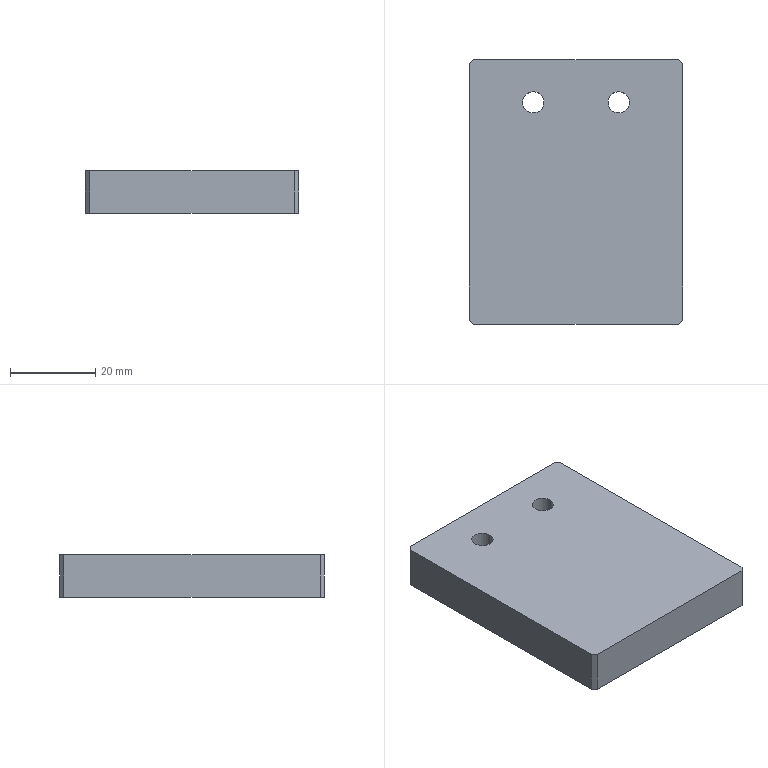Part | STEP file | 2048 Cylinder pad block B | 1 solid | 14 faces | box 50 x 62 x 10 mm | volume 30587 mm3 | plane 10 | cylinder 4 | commonest cylinder face diameters 5 x4
STEP:
#1=CARTESIAN_POINT('',(0.,0.,0.));
#2=DIRECTION('',(0.,0.,1.));
#3=DIRECTION('',(1.,0.,0.));
#4=AXIS2_PLACEMENT_3D('',#1,#2,#3);
#5=CARTESIAN_POINT('',(-7.5,21.,0.));
#6=VERTEX_POINT('',#5);
#7=CARTESIAN_POINT('',(-7.5,21.,10.));
#8=VERTEX_POINT('',#7);
#9=CARTESIAN_POINT('',(-7.5,21.,10.));
#10=DIRECTION('',(0.,0.,1.));
#11=VECTOR('',#10,1.);
#12=LINE('',#9,#11);
#13=CARTESIAN_POINT('',(-10.,21.,10.));
#14=DIRECTION('',(0.,0.,1.));
#15=DIRECTION('',(1.,0.,0.));
#16=AXIS2_PLACEMENT_3D('',#13,#14,#15);
#17=CYLINDRICAL_SURFACE('',#16,2.5);
#18=CARTESIAN_POINT('',(6.283,0.));
#19=DIRECTION('',(0.,1.));
#20=VECTOR('',#19,1.);
#21=LINE('',#18,#20);
#22=(GEOMETRIC_REPRESENTATION_CONTEXT(2)PARAMETRIC_REPRESENTATION_CONTEXT()REPRESENTATION_CONTEXT('',''));
#23=DEFINITIONAL_REPRESENTATION('',(#21),#22);
#24=PCURVE('',#17,#23);
#25=CARTESIAN_POINT('',(-10.,21.,10.));
#26=DIRECTION('',(0.,0.,1.));
#27=DIRECTION('',(1.,0.,0.));
#28=AXIS2_PLACEMENT_3D('',#25,#26,#27);
#29=CYLINDRICAL_SURFACE('',#28,2.5);
#30=CARTESIAN_POINT('',(0.,0.));
#31=DIRECTION('',(0.,1.));
#32=VECTOR('',#31,1.);
#33=LINE('',#30,#32);
#34=(GEOMETRIC_REPRESENTATION_CONTEXT(2)PARAMETRIC_REPRESENTATION_CONTEXT()REPRESENTATION_CONTEXT('',''));
#35=DEFINITIONAL_REPRESENTATION('',(#33),#34);
#36=PCURVE('',#29,#35);
#37=SURFACE_CURVE('',#12,(#24,#36),.PCURVE_S1.);
#38=EDGE_CURVE('',#6,#8,#37,.T.);
#39=ORIENTED_EDGE('',*,*,#38,.T.);
#40=CARTESIAN_POINT('',(-12.5,21.,10.));
#41=VERTEX_POINT('',#40);
#42=CARTESIAN_POINT('',(-10.,21.,10.));
#43=DIRECTION('',(0.,0.,1.));
#44=DIRECTION('',(1.,0.,0.));
#45=AXIS2_PLACEMENT_3D('',#42,#43,#44);
#46=CIRCLE('',#45,2.5);
#47=CARTESIAN_POINT('',(0.,0.));
#48=DIRECTION('',(1.,0.));
#49=VECTOR('',#48,1.);
#50=LINE('',#47,#49);
#51=(GEOMETRIC_REPRESENTATION_CONTEXT(2)PARAMETRIC_REPRESENTATION_CONTEXT()REPRESENTATION_CONTEXT('',''));
#52=DEFINITIONAL_REPRESENTATION('',(#50),#51);
#53=PCURVE('',#17,#52);
#54=CARTESIAN_POINT('',(0.,0.,10.));
#55=DIRECTION('',(0.,0.,-1.));
#56=DIRECTION('',(-1.,0.,0.));
#57=AXIS2_PLACEMENT_3D('',#54,#55,#56);
#58=PLANE('',#57);
#59=CARTESIAN_POINT('',(7.5,21.));
#60=CARTESIAN_POINT('',(7.5,25.33));
#61=CARTESIAN_POINT('',(11.25,23.165));
#62=CARTESIAN_POINT('',(15.,21.));
#63=CARTESIAN_POINT('',(11.25,18.835));
#64=CARTESIAN_POINT('',(7.5,16.67));
#65=CARTESIAN_POINT('',(7.5,21.));
#66=(BOUNDED_CURVE()B_SPLINE_CURVE(2,(#59,#60,#61,#62,#63,#64,#65),.UNSPECIFIED.,.T.,.F.)B_SPLINE_CURVE_WITH_KNOTS((1,2,2,2,2,1),(-2.094,0.,2.094,4.189,6.283,8.378),.UNSPECIFIED.)CURVE()GEOMETRIC_REPRESENTATION_ITEM()RATIONAL_B_SPLINE_CURVE((1.,0.5,1.,0.5,1.,0.5,1.))REPRESENTATION_ITEM(''));
#67=(GEOMETRIC_REPRESENTATION_CONTEXT(2)PARAMETRIC_REPRESENTATION_CONTEXT()REPRESENTATION_CONTEXT('',''));
#68=DEFINITIONAL_REPRESENTATION('',(#66),#67);
#69=PCURVE('',#58,#68);
#70=SURFACE_CURVE('',#46,(#53,#69),.PCURVE_S1.);
#71=EDGE_CURVE('',#41,#8,#70,.T.);
#72=ORIENTED_EDGE('',*,*,#71,.F.);
#73=CARTESIAN_POINT('',(-12.5,21.,0.));
#74=VERTEX_POINT('',#73);
#75=CARTESIAN_POINT('',(-12.5,21.,10.));
#76=DIRECTION('',(0.,0.,1.));
#77=VECTOR('',#76,1.);
#78=LINE('',#75,#77);
#79=CARTESIAN_POINT('',(3.142,0.));
#80=DIRECTION('',(0.,1.));
#81=VECTOR('',#80,1.);
#82=LINE('',#79,#81);
#83=(GEOMETRIC_REPRESENTATION_CONTEXT(2)PARAMETRIC_REPRESENTATION_CONTEXT()REPRESENTATION_CONTEXT('',''));
#84=DEFINITIONAL_REPRESENTATION('',(#82),#83);
#85=PCURVE('',#17,#84);
#86=CARTESIAN_POINT('',(3.142,0.));
#87=DIRECTION('',(0.,1.));
#88=VECTOR('',#87,1.);
#89=LINE('',#86,#88);
#90=(GEOMETRIC_REPRESENTATION_CONTEXT(2)PARAMETRIC_REPRESENTATION_CONTEXT()REPRESENTATION_CONTEXT('',''));
#91=DEFINITIONAL_REPRESENTATION('',(#89),#90);
#92=PCURVE('',#29,#91);
#93=SURFACE_CURVE('',#78,(#85,#92),.PCURVE_S1.);
#94=EDGE_CURVE('',#74,#41,#93,.T.);
#95=ORIENTED_EDGE('',*,*,#94,.F.);
#96=CARTESIAN_POINT('',(-10.,21.,0.));
#97=DIRECTION('',(0.,0.,1.));
#98=DIRECTION('',(1.,0.,0.));
#99=AXIS2_PLACEMENT_3D('',#96,#97,#98);
#100=CIRCLE('',#99,2.5);
#101=CARTESIAN_POINT('',(0.,-10.));
#102=DIRECTION('',(1.,0.));
#103=VECTOR('',#102,1.);
#104=LINE('',#101,#103);
#105=(GEOMETRIC_REPRESENTATION_CONTEXT(2)PARAMETRIC_REPRESENTATION_CONTEXT()REPRESENTATION_CONTEXT('',''));
#106=DEFINITIONAL_REPRESENTATION('',(#104),#105);
#107=PCURVE('',#17,#106);
#108=CARTESIAN_POINT('',(0.,0.,0.));
#109=DIRECTION('',(0.,0.,-1.));
#110=DIRECTION('',(-1.,0.,0.));
#111=AXIS2_PLACEMENT_3D('',#108,#109,#110);
#112=PLANE('',#111);
#113=CARTESIAN_POINT('',(7.5,21.));
#114=CARTESIAN_POINT('',(7.5,25.33));
#115=CARTESIAN_POINT('',(11.25,23.165));
#116=CARTESIAN_POINT('',(15.,21.));
#117=CARTESIAN_POINT('',(11.25,18.835));
#118=CARTESIAN_POINT('',(7.5,16.67));
#119=CARTESIAN_POINT('',(7.5,21.));
#120=(BOUNDED_CURVE()B_SPLINE_CURVE(2,(#113,#114,#115,#116,#117,#118,#119),.UNSPECIFIED.,.T.,.F.)B_SPLINE_CURVE_WITH_KNOTS((1,2,2,2,2,1),(-2.094,0.,2.094,4.189,6.283,8.378),.UNSPECIFIED.)CURVE()GEOMETRIC_REPRESENTATION_ITEM()RATIONAL_B_SPLINE_CURVE((1.,0.5,1.,0.5,1.,0.5,1.))REPRESENTATION_ITEM(''));
#121=(GEOMETRIC_REPRESENTATION_CONTEXT(2)PARAMETRIC_REPRESENTATION_CONTEXT()REPRESENTATION_CONTEXT('',''));
#122=DEFINITIONAL_REPRESENTATION('',(#120),#121);
#123=PCURVE('',#112,#122);
#124=SURFACE_CURVE('',#100,(#107,#123),.PCURVE_S1.);
#125=EDGE_CURVE('',#74,#6,#124,.T.);
#126=ORIENTED_EDGE('',*,*,#125,.T.);
#127=EDGE_LOOP('',(#39,#72,#95,#126));
#128=FACE_BOUND('',#127,.F.);
#129=ADVANCED_FACE('',(#128),#17,.F.);
#130=CARTESIAN_POINT('',(12.5,21.,0.));
#131=VERTEX_POINT('',#130);
#132=CARTESIAN_POINT('',(12.5,21.,10.));
#133=VERTEX_POINT('',#132);
#134=CARTESIAN_POINT('',(12.5,21.,10.));
#135=DIRECTION('',(0.,0.,1.));
#136=VECTOR('',#135,1.);
#137=LINE('',#134,#136);
#138=CARTESIAN_POINT('',(10.,21.,10.));
#139=DIRECTION('',(0.,0.,1.));
#140=DIRECTION('',(1.,0.,0.));
#141=AXIS2_PLACEMENT_3D('',#138,#139,#140);
#142=CYLINDRICAL_SURFACE('',#141,2.5);
#143=CARTESIAN_POINT('',(6.283,0.));
#144=DIRECTION('',(0.,1.));
#145=VECTOR('',#144,1.);
#146=LINE('',#143,#145);
#147=(GEOMETRIC_REPRESENTATION_CONTEXT(2)PARAMETRIC_REPRESENTATION_CONTEXT()REPRESENTATION_CONTEXT('',''));
#148=DEFINITIONAL_REPRESENTATION('',(#146),#147);
#149=PCURVE('',#142,#148);
#150=CARTESIAN_POINT('',(10.,21.,10.));
#151=DIRECTION('',(0.,0.,1.));
#152=DIRECTION('',(1.,0.,0.));
#153=AXIS2_PLACEMENT_3D('',#150,#151,#152);
#154=CYLINDRICAL_SURFACE('',#153,2.5);
#155=CARTESIAN_POINT('',(0.,0.));
#156=DIRECTION('',(0.,1.));
#157=VECTOR('',#156,1.);
#158=LINE('',#155,#157);
#159=(GEOMETRIC_REPRESENTATION_CONTEXT(2)PARAMETRIC_REPRESENTATION_CONTEXT()REPRESENTATION_CONTEXT('',''));
#160=DEFINITIONAL_REPRESENTATION('',(#158),#159);
#161=PCURVE('',#154,#160);
#162=SURFACE_CURVE('',#137,(#149,#161),.PCURVE_S1.);
#163=EDGE_CURVE('',#131,#133,#162,.T.);
#164=ORIENTED_EDGE('',*,*,#163,.T.);
#165=CARTESIAN_POINT('',(7.5,21.,10.));
#166=VERTEX_POINT('',#165);
#167=CARTESIAN_POINT('',(10.,21.,10.));
#168=DIRECTION('',(0.,0.,1.));
#169=DIRECTION('',(1.,0.,0.));
#170=AXIS2_PLACEMENT_3D('',#167,#168,#169);
#171=CIRCLE('',#170,2.5);
#172=CARTESIAN_POINT('',(0.,0.));
#173=DIRECTION('',(1.,0.));
#174=VECTOR('',#173,1.);
#175=LINE('',#172,#174);
#176=(GEOMETRIC_REPRESENTATION_CONTEXT(2)PARAMETRIC_REPRESENTATION_CONTEXT()REPRESENTATION_CONTEXT('',''));
#177=DEFINITIONAL_REPRESENTATION('',(#175),#176);
#178=PCURVE('',#142,#177);
#179=CARTESIAN_POINT('',(-12.5,21.));
#180=CARTESIAN_POINT('',(-12.5,25.33));
#181=CARTESIAN_POINT('',(-8.75,23.165));
#182=CARTESIAN_POINT('',(-5.,21.));
#183=CARTESIAN_POINT('',(-8.75,18.835));
#184=CARTESIAN_POINT('',(-12.5,16.67));
#185=CARTESIAN_POINT('',(-12.5,21.));
#186=(BOUNDED_CURVE()B_SPLINE_CURVE(2,(#179,#180,#181,#182,#183,#184,#185),.UNSPECIFIED.,.T.,.F.)B_SPLINE_CURVE_WITH_KNOTS((1,2,2,2,2,1),(-2.094,0.,2.094,4.189,6.283,8.378),.UNSPECIFIED.)CURVE()GEOMETRIC_REPRESENTATION_ITEM()RATIONAL_B_SPLINE_CURVE((1.,0.5,1.,0.5,1.,0.5,1.))REPRESENTATION_ITEM(''));
#187=(GEOMETRIC_REPRESENTATION_CONTEXT(2)PARAMETRIC_REPRESENTATION_CONTEXT()REPRESENTATION_CONTEXT('',''));
#188=DEFINITIONAL_REPRESENTATION('',(#186),#187);
#189=PCURVE('',#58,#188);
#190=SURFACE_CURVE('',#171,(#178,#189),.PCURVE_S1.);
#191=EDGE_CURVE('',#166,#133,#190,.T.);
#192=ORIENTED_EDGE('',*,*,#191,.F.);
#193=CARTESIAN_POINT('',(7.5,21.,0.));
#194=VERTEX_POINT('',#193);
#195=CARTESIAN_POINT('',(7.5,21.,10.));
#196=DIRECTION('',(0.,0.,1.));
#197=VECTOR('',#196,1.);
#198=LINE('',#195,#197);
#199=CARTESIAN_POINT('',(3.142,0.));
#200=DIRECTION('',(0.,1.));
#201=VECTOR('',#200,1.);
#202=LINE('',#199,#201);
#203=(GEOMETRIC_REPRESENTATION_CONTEXT(2)PARAMETRIC_REPRESENTATION_CONTEXT()REPRESENTATION_CONTEXT('',''));
#204=DEFINITIONAL_REPRESENTATION('',(#202),#203);
#205=PCURVE('',#142,#204);
#206=CARTESIAN_POINT('',(3.142,0.));
#207=DIRECTION('',(0.,1.));
#208=VECTOR('',#207,1.);
#209=LINE('',#206,#208);
#210=(GEOMETRIC_REPRESENTATION_CONTEXT(2)PARAMETRIC_REPRESENTATION_CONTEXT()REPRESENTATION_CONTEXT('',''));
#211=DEFINITIONAL_REPRESENTATION('',(#209),#210);
#212=PCURVE('',#154,#211);
#213=SURFACE_CURVE('',#198,(#205,#212),.PCURVE_S1.);
#214=EDGE_CURVE('',#194,#166,#213,.T.);
#215=ORIENTED_EDGE('',*,*,#214,.F.);
#216=CARTESIAN_POINT('',(10.,21.,0.));
#217=DIRECTION('',(0.,0.,1.));
#218=DIRECTION('',(1.,0.,0.));
#219=AXIS2_PLACEMENT_3D('',#216,#217,#218);
#220=CIRCLE('',#219,2.5);
#221=CARTESIAN_POINT('',(0.,-10.));
#222=DIRECTION('',(1.,0.));
#223=VECTOR('',#222,1.);
#224=LINE('',#221,#223);
#225=(GEOMETRIC_REPRESENTATION_CONTEXT(2)PARAMETRIC_REPRESENTATION_CONTEXT()REPRESENTATION_CONTEXT('',''));
#226=DEFINITIONAL_REPRESENTATION('',(#224),#225);
#227=PCURVE('',#142,#226);
#228=CARTESIAN_POINT('',(-12.5,21.));
#229=CARTESIAN_POINT('',(-12.5,25.33));
#230=CARTESIAN_POINT('',(-8.75,23.165));
#231=CARTESIAN_POINT('',(-5.,21.));
#232=CARTESIAN_POINT('',(-8.75,18.835));
#233=CARTESIAN_POINT('',(-12.5,16.67));
#234=CARTESIAN_POINT('',(-12.5,21.));
#235=(BOUNDED_CURVE()B_SPLINE_CURVE(2,(#228,#229,#230,#231,#232,#233,#234),.UNSPECIFIED.,.T.,.F.)B_SPLINE_CURVE_WITH_KNOTS((1,2,2,2,2,1),(-2.094,0.,2.094,4.189,6.283,8.378),.UNSPECIFIED.)CURVE()GEOMETRIC_REPRESENTATION_ITEM()RATIONAL_B_SPLINE_CURVE((1.,0.5,1.,0.5,1.,0.5,1.))REPRESENTATION_ITEM(''));
#236=(GEOMETRIC_REPRESENTATION_CONTEXT(2)PARAMETRIC_REPRESENTATION_CONTEXT()REPRESENTATION_CONTEXT('',''));
#237=DEFINITIONAL_REPRESENTATION('',(#235),#236);
#238=PCURVE('',#112,#237);
#239=SURFACE_CURVE('',#220,(#227,#238),.PCURVE_S1.);
#240=EDGE_CURVE('',#194,#131,#239,.T.);
#241=ORIENTED_EDGE('',*,*,#240,.T.);
#242=EDGE_LOOP('',(#164,#192,#215,#241));
#243=FACE_BOUND('',#242,.F.);
#244=ADVANCED_FACE('',(#243),#142,.F.);
#245=CARTESIAN_POINT('',(25.,-30.,10.));
#246=VERTEX_POINT('',#245);
#247=CARTESIAN_POINT('',(25.,30.,10.));
#248=VERTEX_POINT('',#247);
#249=CARTESIAN_POINT('',(25.,-31.,10.));
#250=DIRECTION('',(0.,1.,0.));
#251=VECTOR('',#250,1.);
#252=LINE('',#249,#251);
#253=CARTESIAN_POINT('',(25.,-31.,10.));
#254=DIRECTION('',(-1.,0.,0.));
#255=DIRECTION('',(0.,0.,1.));
#256=AXIS2_PLACEMENT_3D('',#253,#254,#255);
#257=PLANE('',#256);
#258=CARTESIAN_POINT('',(0.,0.));
#259=DIRECTION('',(0.,1.));
#260=VECTOR('',#259,1.);
#261=LINE('',#258,#260);
#262=(GEOMETRIC_REPRESENTATION_CONTEXT(2)PARAMETRIC_REPRESENTATION_CONTEXT()REPRESENTATION_CONTEXT('',''));
#263=DEFINITIONAL_REPRESENTATION('',(#261),#262);
#264=PCURVE('',#257,#263);
#265=CARTESIAN_POINT('',(-25.,-31.));
#266=DIRECTION('',(0.,1.));
#267=VECTOR('',#266,1.);
#268=LINE('',#265,#267);
#269=(GEOMETRIC_REPRESENTATION_CONTEXT(2)PARAMETRIC_REPRESENTATION_CONTEXT()REPRESENTATION_CONTEXT('',''));
#270=DEFINITIONAL_REPRESENTATION('',(#268),#269);
#271=PCURVE('',#58,#270);
#272=SURFACE_CURVE('',#252,(#264,#271),.PCURVE_S1.);
#273=EDGE_CURVE('',#246,#248,#272,.T.);
#274=ORIENTED_EDGE('',*,*,#273,.F.);
#275=CARTESIAN_POINT('',(25.,-30.,0.));
#276=VERTEX_POINT('',#275);
#277=CARTESIAN_POINT('',(25.,-30.,10.));
#278=DIRECTION('',(0.,0.,-1.));
#279=VECTOR('',#278,1.);
#280=LINE('',#277,#279);
#281=CARTESIAN_POINT('',(0.,1.));
#282=DIRECTION('',(-1.,0.));
#283=VECTOR('',#282,1.);
#284=LINE('',#281,#283);
#285=(GEOMETRIC_REPRESENTATION_CONTEXT(2)PARAMETRIC_REPRESENTATION_CONTEXT()REPRESENTATION_CONTEXT('',''));
#286=DEFINITIONAL_REPRESENTATION('',(#284),#285);
#287=PCURVE('',#257,#286);
#288=CARTESIAN_POINT('',(25.,-30.,10.));
#289=DIRECTION('',(-0.7071,0.7071,0.));
#290=DIRECTION('',(0.,0.,-1.));
#291=AXIS2_PLACEMENT_3D('',#288,#289,#290);
#292=PLANE('',#291);
#293=CARTESIAN_POINT('',(0.,0.));
#294=DIRECTION('',(1.,0.));
#295=VECTOR('',#294,1.);
#296=LINE('',#293,#295);
#297=(GEOMETRIC_REPRESENTATION_CONTEXT(2)PARAMETRIC_REPRESENTATION_CONTEXT()REPRESENTATION_CONTEXT('',''));
#298=DEFINITIONAL_REPRESENTATION('',(#296),#297);
#299=PCURVE('',#292,#298);
#300=SURFACE_CURVE('',#280,(#287,#299),.PCURVE_S1.);
#301=EDGE_CURVE('',#246,#276,#300,.T.);
#302=ORIENTED_EDGE('',*,*,#301,.T.);
#303=CARTESIAN_POINT('',(25.,30.,0.));
#304=VERTEX_POINT('',#303);
#305=CARTESIAN_POINT('',(25.,-31.,0.));
#306=DIRECTION('',(0.,1.,0.));
#307=VECTOR('',#306,1.);
#308=LINE('',#305,#307);
#309=CARTESIAN_POINT('',(-10.,0.));
#310=DIRECTION('',(0.,1.));
#311=VECTOR('',#310,1.);
#312=LINE('',#309,#311);
#313=(GEOMETRIC_REPRESENTATION_CONTEXT(2)PARAMETRIC_REPRESENTATION_CONTEXT()REPRESENTATION_CONTEXT('',''));
#314=DEFINITIONAL_REPRESENTATION('',(#312),#313);
#315=PCURVE('',#257,#314);
#316=CARTESIAN_POINT('',(-25.,-31.));
#317=DIRECTION('',(0.,1.));
#318=VECTOR('',#317,1.);
#319=LINE('',#316,#318);
#320=(GEOMETRIC_REPRESENTATION_CONTEXT(2)PARAMETRIC_REPRESENTATION_CONTEXT()REPRESENTATION_CONTEXT('',''));
#321=DEFINITIONAL_REPRESENTATION('',(#319),#320);
#322=PCURVE('',#112,#321);
#323=SURFACE_CURVE('',#308,(#315,#322),.PCURVE_S1.);
#324=EDGE_CURVE('',#276,#304,#323,.T.);
#325=ORIENTED_EDGE('',*,*,#324,.T.);
#326=CARTESIAN_POINT('',(25.,30.,10.));
#327=DIRECTION('',(0.,0.,1.));
#328=VECTOR('',#327,1.);
#329=LINE('',#326,#328);
#330=CARTESIAN_POINT('',(0.,61.));
#331=DIRECTION('',(1.,0.));
#332=VECTOR('',#331,1.);
#333=LINE('',#330,#332);
#334=(GEOMETRIC_REPRESENTATION_CONTEXT(2)PARAMETRIC_REPRESENTATION_CONTEXT()REPRESENTATION_CONTEXT('',''));
#335=DEFINITIONAL_REPRESENTATION('',(#333),#334);
#336=PCURVE('',#257,#335);
#337=CARTESIAN_POINT('',(24.,31.,10.));
#338=DIRECTION('',(-0.7071,-0.7071,0.));
#339=DIRECTION('',(0.,0.,-1.));
#340=AXIS2_PLACEMENT_3D('',#337,#338,#339);
#341=PLANE('',#340);
#342=CARTESIAN_POINT('',(0.,1.414));
#343=DIRECTION('',(-1.,0.));
#344=VECTOR('',#343,1.);
#345=LINE('',#342,#344);
#346=(GEOMETRIC_REPRESENTATION_CONTEXT(2)PARAMETRIC_REPRESENTATION_CONTEXT()REPRESENTATION_CONTEXT('',''));
#347=DEFINITIONAL_REPRESENTATION('',(#345),#346);
#348=PCURVE('',#341,#347);
#349=SURFACE_CURVE('',#329,(#336,#348),.PCURVE_S1.);
#350=EDGE_CURVE('',#304,#248,#349,.T.);
#351=ORIENTED_EDGE('',*,*,#350,.T.);
#352=EDGE_LOOP('',(#274,#302,#325,#351));
#353=FACE_BOUND('',#352,.T.);
#354=ADVANCED_FACE('',(#353),#257,.F.);
#355=CARTESIAN_POINT('',(24.,31.,10.));
#356=VERTEX_POINT('',#355);
#357=CARTESIAN_POINT('',(-24.,31.,10.));
#358=VERTEX_POINT('',#357);
#359=CARTESIAN_POINT('',(-25.,31.,10.));
#360=DIRECTION('',(-1.,0.,0.));
#361=VECTOR('',#360,1.);
#362=LINE('',#359,#361);
#363=CARTESIAN_POINT('',(-25.,31.,10.));
#364=DIRECTION('',(0.,-1.,0.));
#365=DIRECTION('',(0.,0.,-1.));
#366=AXIS2_PLACEMENT_3D('',#363,#364,#365);
#367=PLANE('',#366);
#368=CARTESIAN_POINT('',(0.,0.));
#369=DIRECTION('',(0.,-1.));
#370=VECTOR('',#369,1.);
#371=LINE('',#368,#370);
#372=(GEOMETRIC_REPRESENTATION_CONTEXT(2)PARAMETRIC_REPRESENTATION_CONTEXT()REPRESENTATION_CONTEXT('',''));
#373=DEFINITIONAL_REPRESENTATION('',(#371),#372);
#374=PCURVE('',#367,#373);
#375=CARTESIAN_POINT('',(25.,31.));
#376=DIRECTION('',(1.,0.));
#377=VECTOR('',#376,1.);
#378=LINE('',#375,#377);
#379=(GEOMETRIC_REPRESENTATION_CONTEXT(2)PARAMETRIC_REPRESENTATION_CONTEXT()REPRESENTATION_CONTEXT('',''));
#380=DEFINITIONAL_REPRESENTATION('',(#378),#379);
#381=PCURVE('',#58,#380);
#382=SURFACE_CURVE('',#362,(#374,#381),.PCURVE_S1.);
#383=EDGE_CURVE('',#356,#358,#382,.T.);
#384=ORIENTED_EDGE('',*,*,#383,.F.);
#385=CARTESIAN_POINT('',(24.,31.,0.));
#386=VERTEX_POINT('',#385);
#387=CARTESIAN_POINT('',(24.,31.,10.));
#388=DIRECTION('',(0.,0.,-1.));
#389=VECTOR('',#388,1.);
#390=LINE('',#387,#389);
#391=CARTESIAN_POINT('',(0.,49.));
#392=DIRECTION('',(1.,0.));
#393=VECTOR('',#392,1.);
#394=LINE('',#391,#393);
#395=(GEOMETRIC_REPRESENTATION_CONTEXT(2)PARAMETRIC_REPRESENTATION_CONTEXT()REPRESENTATION_CONTEXT('',''));
#396=DEFINITIONAL_REPRESENTATION('',(#394),#395);
#397=PCURVE('',#367,#396);
#398=CARTESIAN_POINT('',(0.,0.));
#399=DIRECTION('',(1.,0.));
#400=VECTOR('',#399,1.);
#401=LINE('',#398,#400);
#402=(GEOMETRIC_REPRESENTATION_CONTEXT(2)PARAMETRIC_REPRESENTATION_CONTEXT()REPRESENTATION_CONTEXT('',''));
#403=DEFINITIONAL_REPRESENTATION('',(#401),#402);
#404=PCURVE('',#341,#403);
#405=SURFACE_CURVE('',#390,(#397,#404),.PCURVE_S1.);
#406=EDGE_CURVE('',#356,#386,#405,.T.);
#407=ORIENTED_EDGE('',*,*,#406,.T.);
#408=CARTESIAN_POINT('',(-24.,31.,0.));
#409=VERTEX_POINT('',#408);
#410=CARTESIAN_POINT('',(-25.,31.,0.));
#411=DIRECTION('',(-1.,0.,0.));
#412=VECTOR('',#411,1.);
#413=LINE('',#410,#412);
#414=CARTESIAN_POINT('',(10.,0.));
#415=DIRECTION('',(0.,-1.));
#416=VECTOR('',#415,1.);
#417=LINE('',#414,#416);
#418=(GEOMETRIC_REPRESENTATION_CONTEXT(2)PARAMETRIC_REPRESENTATION_CONTEXT()REPRESENTATION_CONTEXT('',''));
#419=DEFINITIONAL_REPRESENTATION('',(#417),#418);
#420=PCURVE('',#367,#419);
#421=CARTESIAN_POINT('',(25.,31.));
#422=DIRECTION('',(1.,0.));
#423=VECTOR('',#422,1.);
#424=LINE('',#421,#423);
#425=(GEOMETRIC_REPRESENTATION_CONTEXT(2)PARAMETRIC_REPRESENTATION_CONTEXT()REPRESENTATION_CONTEXT('',''));
#426=DEFINITIONAL_REPRESENTATION('',(#424),#425);
#427=PCURVE('',#112,#426);
#428=SURFACE_CURVE('',#413,(#420,#427),.PCURVE_S1.);
#429=EDGE_CURVE('',#386,#409,#428,.T.);
#430=ORIENTED_EDGE('',*,*,#429,.T.);
#431=CARTESIAN_POINT('',(-24.,31.,10.));
#432=DIRECTION('',(0.,0.,1.));
#433=VECTOR('',#432,1.);
#434=LINE('',#431,#433);
#435=CARTESIAN_POINT('',(0.,1.));
#436=DIRECTION('',(-1.,0.));
#437=VECTOR('',#436,1.);
#438=LINE('',#435,#437);
#439=(GEOMETRIC_REPRESENTATION_CONTEXT(2)PARAMETRIC_REPRESENTATION_CONTEXT()REPRESENTATION_CONTEXT('',''));
#440=DEFINITIONAL_REPRESENTATION('',(#438),#439);
#441=PCURVE('',#367,#440);
#442=CARTESIAN_POINT('',(-25.,30.,10.));
#443=DIRECTION('',(0.7071,-0.7071,0.));
#444=DIRECTION('',(0.,0.,-1.));
#445=AXIS2_PLACEMENT_3D('',#442,#443,#444);
#446=PLANE('',#445);
#447=CARTESIAN_POINT('',(0.,1.414));
#448=DIRECTION('',(-1.,0.));
#449=VECTOR('',#448,1.);
#450=LINE('',#447,#449);
#451=(GEOMETRIC_REPRESENTATION_CONTEXT(2)PARAMETRIC_REPRESENTATION_CONTEXT()REPRESENTATION_CONTEXT('',''));
#452=DEFINITIONAL_REPRESENTATION('',(#450),#451);
#453=PCURVE('',#446,#452);
#454=SURFACE_CURVE('',#434,(#441,#453),.PCURVE_S1.);
#455=EDGE_CURVE('',#409,#358,#454,.T.);
#456=ORIENTED_EDGE('',*,*,#455,.T.);
#457=EDGE_LOOP('',(#384,#407,#430,#456));
#458=FACE_BOUND('',#457,.T.);
#459=ADVANCED_FACE('',(#458),#367,.F.);
#460=CARTESIAN_POINT('',(-25.,30.,0.));
#461=VERTEX_POINT('',#460);
#462=CARTESIAN_POINT('',(-25.,-30.,0.));
#463=VERTEX_POINT('',#462);
#464=CARTESIAN_POINT('',(-25.,-31.,0.));
#465=DIRECTION('',(0.,-1.,0.));
#466=VECTOR('',#465,1.);
#467=LINE('',#464,#466);
#468=CARTESIAN_POINT('',(-25.,-31.,10.));
#469=DIRECTION('',(1.,0.,0.));
#470=DIRECTION('',(0.,0.,-1.));
#471=AXIS2_PLACEMENT_3D('',#468,#469,#470);
#472=PLANE('',#471);
#473=CARTESIAN_POINT('',(10.,0.));
#474=DIRECTION('',(0.,-1.));
#475=VECTOR('',#474,1.);
#476=LINE('',#473,#475);
#477=(GEOMETRIC_REPRESENTATION_CONTEXT(2)PARAMETRIC_REPRESENTATION_CONTEXT()REPRESENTATION_CONTEXT('',''));
#478=DEFINITIONAL_REPRESENTATION('',(#476),#477);
#479=PCURVE('',#472,#478);
#480=CARTESIAN_POINT('',(25.,-31.));
#481=DIRECTION('',(0.,-1.));
#482=VECTOR('',#481,1.);
#483=LINE('',#480,#482);
#484=(GEOMETRIC_REPRESENTATION_CONTEXT(2)PARAMETRIC_REPRESENTATION_CONTEXT()REPRESENTATION_CONTEXT('',''));
#485=DEFINITIONAL_REPRESENTATION('',(#483),#484);
#486=PCURVE('',#112,#485);
#487=SURFACE_CURVE('',#467,(#479,#486),.PCURVE_S1.);
#488=EDGE_CURVE('',#461,#463,#487,.T.);
#489=ORIENTED_EDGE('',*,*,#488,.T.);
#490=CARTESIAN_POINT('',(-25.,-30.,10.));
#491=VERTEX_POINT('',#490);
#492=CARTESIAN_POINT('',(-25.,-30.,10.));
#493=DIRECTION('',(0.,0.,1.));
#494=VECTOR('',#493,1.);
#495=LINE('',#492,#494);
#496=CARTESIAN_POINT('',(0.,1.));
#497=DIRECTION('',(-1.,0.));
#498=VECTOR('',#497,1.);
#499=LINE('',#496,#498);
#500=(GEOMETRIC_REPRESENTATION_CONTEXT(2)PARAMETRIC_REPRESENTATION_CONTEXT()REPRESENTATION_CONTEXT('',''));
#501=DEFINITIONAL_REPRESENTATION('',(#499),#500);
#502=PCURVE('',#472,#501);
#503=CARTESIAN_POINT('',(-24.,-31.,10.));
#504=DIRECTION('',(0.7071,0.7071,0.));
#505=DIRECTION('',(0.,0.,-1.));
#506=AXIS2_PLACEMENT_3D('',#503,#504,#505);
#507=PLANE('',#506);
#508=CARTESIAN_POINT('',(0.,1.414));
#509=DIRECTION('',(-1.,0.));
#510=VECTOR('',#509,1.);
#511=LINE('',#508,#510);
#512=(GEOMETRIC_REPRESENTATION_CONTEXT(2)PARAMETRIC_REPRESENTATION_CONTEXT()REPRESENTATION_CONTEXT('',''));
#513=DEFINITIONAL_REPRESENTATION('',(#511),#512);
#514=PCURVE('',#507,#513);
#515=SURFACE_CURVE('',#495,(#502,#514),.PCURVE_S1.);
#516=EDGE_CURVE('',#463,#491,#515,.T.);
#517=ORIENTED_EDGE('',*,*,#516,.T.);
#518=CARTESIAN_POINT('',(-25.,30.,10.));
#519=VERTEX_POINT('',#518);
#520=CARTESIAN_POINT('',(-25.,-31.,10.));
#521=DIRECTION('',(0.,-1.,0.));
#522=VECTOR('',#521,1.);
#523=LINE('',#520,#522);
#524=CARTESIAN_POINT('',(0.,0.));
#525=DIRECTION('',(0.,-1.));
#526=VECTOR('',#525,1.);
#527=LINE('',#524,#526);
#528=(GEOMETRIC_REPRESENTATION_CONTEXT(2)PARAMETRIC_REPRESENTATION_CONTEXT()REPRESENTATION_CONTEXT('',''));
#529=DEFINITIONAL_REPRESENTATION('',(#527),#528);
#530=PCURVE('',#472,#529);
#531=CARTESIAN_POINT('',(25.,-31.));
#532=DIRECTION('',(0.,-1.));
#533=VECTOR('',#532,1.);
#534=LINE('',#531,#533);
#535=(GEOMETRIC_REPRESENTATION_CONTEXT(2)PARAMETRIC_REPRESENTATION_CONTEXT()REPRESENTATION_CONTEXT('',''));
#536=DEFINITIONAL_REPRESENTATION('',(#534),#535);
#537=PCURVE('',#58,#536);
#538=SURFACE_CURVE('',#523,(#530,#537),.PCURVE_S1.);
#539=EDGE_CURVE('',#519,#491,#538,.T.);
#540=ORIENTED_EDGE('',*,*,#539,.F.);
#541=CARTESIAN_POINT('',(-25.,30.,10.));
#542=DIRECTION('',(0.,0.,-1.));
#543=VECTOR('',#542,1.);
#544=LINE('',#541,#543);
#545=CARTESIAN_POINT('',(0.,61.));
#546=DIRECTION('',(1.,0.));
#547=VECTOR('',#546,1.);
#548=LINE('',#545,#547);
#549=(GEOMETRIC_REPRESENTATION_CONTEXT(2)PARAMETRIC_REPRESENTATION_CONTEXT()REPRESENTATION_CONTEXT('',''));
#550=DEFINITIONAL_REPRESENTATION('',(#548),#549);
#551=PCURVE('',#472,#550);
#552=CARTESIAN_POINT('',(0.,0.));
#553=DIRECTION('',(1.,0.));
#554=VECTOR('',#553,1.);
#555=LINE('',#552,#554);
#556=(GEOMETRIC_REPRESENTATION_CONTEXT(2)PARAMETRIC_REPRESENTATION_CONTEXT()REPRESENTATION_CONTEXT('',''));
#557=DEFINITIONAL_REPRESENTATION('',(#555),#556);
#558=PCURVE('',#446,#557);
#559=SURFACE_CURVE('',#544,(#551,#558),.PCURVE_S1.);
#560=EDGE_CURVE('',#519,#461,#559,.T.);
#561=ORIENTED_EDGE('',*,*,#560,.T.);
#562=EDGE_LOOP('',(#489,#517,#540,#561));
#563=FACE_BOUND('',#562,.T.);
#564=ADVANCED_FACE('',(#563),#472,.F.);
#565=CARTESIAN_POINT('',(-24.,-31.,10.));
#566=VERTEX_POINT('',#565);
#567=CARTESIAN_POINT('',(24.,-31.,10.));
#568=VERTEX_POINT('',#567);
#569=CARTESIAN_POINT('',(-25.,-31.,10.));
#570=DIRECTION('',(1.,0.,0.));
#571=VECTOR('',#570,1.);
#572=LINE('',#569,#571);
#573=CARTESIAN_POINT('',(-25.,-31.,10.));
#574=DIRECTION('',(0.,1.,0.));
#575=DIRECTION('',(0.,0.,1.));
#576=AXIS2_PLACEMENT_3D('',#573,#574,#575);
#577=PLANE('',#576);
#578=CARTESIAN_POINT('',(0.,0.));
#579=DIRECTION('',(0.,1.));
#580=VECTOR('',#579,1.);
#581=LINE('',#578,#580);
#582=(GEOMETRIC_REPRESENTATION_CONTEXT(2)PARAMETRIC_REPRESENTATION_CONTEXT()REPRESENTATION_CONTEXT('',''));
#583=DEFINITIONAL_REPRESENTATION('',(#581),#582);
#584=PCURVE('',#577,#583);
#585=CARTESIAN_POINT('',(25.,-31.));
#586=DIRECTION('',(-1.,0.));
#587=VECTOR('',#586,1.);
#588=LINE('',#585,#587);
#589=(GEOMETRIC_REPRESENTATION_CONTEXT(2)PARAMETRIC_REPRESENTATION_CONTEXT()REPRESENTATION_CONTEXT('',''));
#590=DEFINITIONAL_REPRESENTATION('',(#588),#589);
#591=PCURVE('',#58,#590);
#592=SURFACE_CURVE('',#572,(#584,#591),.PCURVE_S1.);
#593=EDGE_CURVE('',#566,#568,#592,.T.);
#594=ORIENTED_EDGE('',*,*,#593,.F.);
#595=CARTESIAN_POINT('',(-24.,-31.,0.));
#596=VERTEX_POINT('',#595);
#597=CARTESIAN_POINT('',(-24.,-31.,10.));
#598=DIRECTION('',(0.,0.,-1.));
#599=VECTOR('',#598,1.);
#600=LINE('',#597,#599);
#601=CARTESIAN_POINT('',(0.,1.));
#602=DIRECTION('',(-1.,0.));
#603=VECTOR('',#602,1.);
#604=LINE('',#601,#603);
#605=(GEOMETRIC_REPRESENTATION_CONTEXT(2)PARAMETRIC_REPRESENTATION_CONTEXT()REPRESENTATION_CONTEXT('',''));
#606=DEFINITIONAL_REPRESENTATION('',(#604),#605);
#607=PCURVE('',#577,#606);
#608=CARTESIAN_POINT('',(0.,0.));
#609=DIRECTION('',(1.,0.));
#610=VECTOR('',#609,1.);
#611=LINE('',#608,#610);
#612=(GEOMETRIC_REPRESENTATION_CONTEXT(2)PARAMETRIC_REPRESENTATION_CONTEXT()REPRESENTATION_CONTEXT('',''));
#613=DEFINITIONAL_REPRESENTATION('',(#611),#612);
#614=PCURVE('',#507,#613);
#615=SURFACE_CURVE('',#600,(#607,#614),.PCURVE_S1.);
#616=EDGE_CURVE('',#566,#596,#615,.T.);
#617=ORIENTED_EDGE('',*,*,#616,.T.);
#618=CARTESIAN_POINT('',(24.,-31.,0.));
#619=VERTEX_POINT('',#618);
#620=CARTESIAN_POINT('',(-25.,-31.,0.));
#621=DIRECTION('',(1.,0.,0.));
#622=VECTOR('',#621,1.);
#623=LINE('',#620,#622);
#624=CARTESIAN_POINT('',(-10.,0.));
#625=DIRECTION('',(0.,1.));
#626=VECTOR('',#625,1.);
#627=LINE('',#624,#626);
#628=(GEOMETRIC_REPRESENTATION_CONTEXT(2)PARAMETRIC_REPRESENTATION_CONTEXT()REPRESENTATION_CONTEXT('',''));
#629=DEFINITIONAL_REPRESENTATION('',(#627),#628);
#630=PCURVE('',#577,#629);
#631=CARTESIAN_POINT('',(25.,-31.));
#632=DIRECTION('',(-1.,0.));
#633=VECTOR('',#632,1.);
#634=LINE('',#631,#633);
#635=(GEOMETRIC_REPRESENTATION_CONTEXT(2)PARAMETRIC_REPRESENTATION_CONTEXT()REPRESENTATION_CONTEXT('',''));
#636=DEFINITIONAL_REPRESENTATION('',(#634),#635);
#637=PCURVE('',#112,#636);
#638=SURFACE_CURVE('',#623,(#630,#637),.PCURVE_S1.);
#639=EDGE_CURVE('',#596,#619,#638,.T.);
#640=ORIENTED_EDGE('',*,*,#639,.T.);
#641=CARTESIAN_POINT('',(24.,-31.,10.));
#642=DIRECTION('',(0.,0.,1.));
#643=VECTOR('',#642,1.);
#644=LINE('',#641,#643);
#645=CARTESIAN_POINT('',(0.,49.));
#646=DIRECTION('',(1.,0.));
#647=VECTOR('',#646,1.);
#648=LINE('',#645,#647);
#649=(GEOMETRIC_REPRESENTATION_CONTEXT(2)PARAMETRIC_REPRESENTATION_CONTEXT()REPRESENTATION_CONTEXT('',''));
#650=DEFINITIONAL_REPRESENTATION('',(#648),#649);
#651=PCURVE('',#577,#650);
#652=CARTESIAN_POINT('',(0.,1.414));
#653=DIRECTION('',(-1.,0.));
#654=VECTOR('',#653,1.);
#655=LINE('',#652,#654);
#656=(GEOMETRIC_REPRESENTATION_CONTEXT(2)PARAMETRIC_REPRESENTATION_CONTEXT()REPRESENTATION_CONTEXT('',''));
#657=DEFINITIONAL_REPRESENTATION('',(#655),#656);
#658=PCURVE('',#292,#657);
#659=SURFACE_CURVE('',#644,(#651,#658),.PCURVE_S1.);
#660=EDGE_CURVE('',#619,#568,#659,.T.);
#661=ORIENTED_EDGE('',*,*,#660,.T.);
#662=EDGE_LOOP('',(#594,#617,#640,#661));
#663=FACE_BOUND('',#662,.T.);
#664=ADVANCED_FACE('',(#663),#577,.F.);
#665=CARTESIAN_POINT('',(-10.,21.,10.));
#666=DIRECTION('',(0.,0.,1.));
#667=DIRECTION('',(1.,0.,0.));
#668=AXIS2_PLACEMENT_3D('',#665,#666,#667);
#669=CIRCLE('',#668,2.5);
#670=CARTESIAN_POINT('',(7.5,21.));
#671=CARTESIAN_POINT('',(7.5,25.33));
#672=CARTESIAN_POINT('',(11.25,23.165));
#673=CARTESIAN_POINT('',(15.,21.));
#674=CARTESIAN_POINT('',(11.25,18.835));
#675=CARTESIAN_POINT('',(7.5,16.67));
#676=CARTESIAN_POINT('',(7.5,21.));
#677=(BOUNDED_CURVE()B_SPLINE_CURVE(2,(#670,#671,#672,#673,#674,#675,#676),.UNSPECIFIED.,.T.,.F.)B_SPLINE_CURVE_WITH_KNOTS((1,2,2,2,2,1),(-2.094,0.,2.094,4.189,6.283,8.378),.UNSPECIFIED.)CURVE()GEOMETRIC_REPRESENTATION_ITEM()RATIONAL_B_SPLINE_CURVE((1.,0.5,1.,0.5,1.,0.5,1.))REPRESENTATION_ITEM(''));
#678=(GEOMETRIC_REPRESENTATION_CONTEXT(2)PARAMETRIC_REPRESENTATION_CONTEXT()REPRESENTATION_CONTEXT('',''));
#679=DEFINITIONAL_REPRESENTATION('',(#677),#678);
#680=PCURVE('',#58,#679);
#681=CARTESIAN_POINT('',(0.,0.));
#682=DIRECTION('',(1.,0.));
#683=VECTOR('',#682,1.);
#684=LINE('',#681,#683);
#685=(GEOMETRIC_REPRESENTATION_CONTEXT(2)PARAMETRIC_REPRESENTATION_CONTEXT()REPRESENTATION_CONTEXT('',''));
#686=DEFINITIONAL_REPRESENTATION('',(#684),#685);
#687=PCURVE('',#29,#686);
#688=SURFACE_CURVE('',#669,(#680,#687),.PCURVE_S1.);
#689=EDGE_CURVE('',#8,#41,#688,.T.);
#690=ORIENTED_EDGE('',*,*,#689,.F.);
#691=ORIENTED_EDGE('',*,*,#71,.F.);
#692=EDGE_LOOP('',(#690,#691));
#693=FACE_BOUND('',#692,.T.);
#694=CARTESIAN_POINT('',(10.,21.,10.));
#695=DIRECTION('',(0.,0.,1.));
#696=DIRECTION('',(1.,0.,0.));
#697=AXIS2_PLACEMENT_3D('',#694,#695,#696);
#698=CIRCLE('',#697,2.5);
#699=CARTESIAN_POINT('',(-12.5,21.));
#700=CARTESIAN_POINT('',(-12.5,25.33));
#701=CARTESIAN_POINT('',(-8.75,23.165));
#702=CARTESIAN_POINT('',(-5.,21.));
#703=CARTESIAN_POINT('',(-8.75,18.835));
#704=CARTESIAN_POINT('',(-12.5,16.67));
#705=CARTESIAN_POINT('',(-12.5,21.));
#706=(BOUNDED_CURVE()B_SPLINE_CURVE(2,(#699,#700,#701,#702,#703,#704,#705),.UNSPECIFIED.,.T.,.F.)B_SPLINE_CURVE_WITH_KNOTS((1,2,2,2,2,1),(-2.094,0.,2.094,4.189,6.283,8.378),.UNSPECIFIED.)CURVE()GEOMETRIC_REPRESENTATION_ITEM()RATIONAL_B_SPLINE_CURVE((1.,0.5,1.,0.5,1.,0.5,1.))REPRESENTATION_ITEM(''));
#707=(GEOMETRIC_REPRESENTATION_CONTEXT(2)PARAMETRIC_REPRESENTATION_CONTEXT()REPRESENTATION_CONTEXT('',''));
#708=DEFINITIONAL_REPRESENTATION('',(#706),#707);
#709=PCURVE('',#58,#708);
#710=CARTESIAN_POINT('',(0.,0.));
#711=DIRECTION('',(1.,0.));
#712=VECTOR('',#711,1.);
#713=LINE('',#710,#712);
#714=(GEOMETRIC_REPRESENTATION_CONTEXT(2)PARAMETRIC_REPRESENTATION_CONTEXT()REPRESENTATION_CONTEXT('',''));
#715=DEFINITIONAL_REPRESENTATION('',(#713),#714);
#716=PCURVE('',#154,#715);
#717=SURFACE_CURVE('',#698,(#709,#716),.PCURVE_S1.);
#718=EDGE_CURVE('',#133,#166,#717,.T.);
#719=ORIENTED_EDGE('',*,*,#718,.F.);
#720=ORIENTED_EDGE('',*,*,#191,.F.);
#721=EDGE_LOOP('',(#719,#720));
#722=FACE_BOUND('',#721,.T.);
#723=ORIENTED_EDGE('',*,*,#539,.T.);
#724=CARTESIAN_POINT('',(-24.,-31.,10.));
#725=DIRECTION('',(0.7071,-0.7071,0.));
#726=VECTOR('',#725,1.);
#727=LINE('',#724,#726);
#728=CARTESIAN_POINT('',(24.,-31.));
#729=DIRECTION('',(-0.7071,-0.7071));
#730=VECTOR('',#729,1.);
#731=LINE('',#728,#730);
#732=(GEOMETRIC_REPRESENTATION_CONTEXT(2)PARAMETRIC_REPRESENTATION_CONTEXT()REPRESENTATION_CONTEXT('',''));
#733=DEFINITIONAL_REPRESENTATION('',(#731),#732);
#734=PCURVE('',#58,#733);
#735=CARTESIAN_POINT('',(0.,0.));
#736=DIRECTION('',(0.,-1.));
#737=VECTOR('',#736,1.);
#738=LINE('',#735,#737);
#739=(GEOMETRIC_REPRESENTATION_CONTEXT(2)PARAMETRIC_REPRESENTATION_CONTEXT()REPRESENTATION_CONTEXT('',''));
#740=DEFINITIONAL_REPRESENTATION('',(#738),#739);
#741=PCURVE('',#507,#740);
#742=SURFACE_CURVE('',#727,(#734,#741),.PCURVE_S1.);
#743=EDGE_CURVE('',#491,#566,#742,.T.);
#744=ORIENTED_EDGE('',*,*,#743,.T.);
#745=ORIENTED_EDGE('',*,*,#593,.T.);
#746=CARTESIAN_POINT('',(25.,-30.,10.));
#747=DIRECTION('',(0.7071,0.7071,0.));
#748=VECTOR('',#747,1.);
#749=LINE('',#746,#748);
#750=CARTESIAN_POINT('',(-25.,-30.));
#751=DIRECTION('',(-0.7071,0.7071));
#752=VECTOR('',#751,1.);
#753=LINE('',#750,#752);
#754=(GEOMETRIC_REPRESENTATION_CONTEXT(2)PARAMETRIC_REPRESENTATION_CONTEXT()REPRESENTATION_CONTEXT('',''));
#755=DEFINITIONAL_REPRESENTATION('',(#753),#754);
#756=PCURVE('',#58,#755);
#757=CARTESIAN_POINT('',(0.,0.));
#758=DIRECTION('',(0.,-1.));
#759=VECTOR('',#758,1.);
#760=LINE('',#757,#759);
#761=(GEOMETRIC_REPRESENTATION_CONTEXT(2)PARAMETRIC_REPRESENTATION_CONTEXT()REPRESENTATION_CONTEXT('',''));
#762=DEFINITIONAL_REPRESENTATION('',(#760),#761);
#763=PCURVE('',#292,#762);
#764=SURFACE_CURVE('',#749,(#756,#763),.PCURVE_S1.);
#765=EDGE_CURVE('',#568,#246,#764,.T.);
#766=ORIENTED_EDGE('',*,*,#765,.T.);
#767=ORIENTED_EDGE('',*,*,#273,.T.);
#768=CARTESIAN_POINT('',(24.,31.,10.));
#769=DIRECTION('',(-0.7071,0.7071,0.));
#770=VECTOR('',#769,1.);
#771=LINE('',#768,#770);
#772=CARTESIAN_POINT('',(-24.,31.));
#773=DIRECTION('',(0.7071,0.7071));
#774=VECTOR('',#773,1.);
#775=LINE('',#772,#774);
#776=(GEOMETRIC_REPRESENTATION_CONTEXT(2)PARAMETRIC_REPRESENTATION_CONTEXT()REPRESENTATION_CONTEXT('',''));
#777=DEFINITIONAL_REPRESENTATION('',(#775),#776);
#778=PCURVE('',#58,#777);
#779=CARTESIAN_POINT('',(0.,0.));
#780=DIRECTION('',(0.,-1.));
#781=VECTOR('',#780,1.);
#782=LINE('',#779,#781);
#783=(GEOMETRIC_REPRESENTATION_CONTEXT(2)PARAMETRIC_REPRESENTATION_CONTEXT()REPRESENTATION_CONTEXT('',''));
#784=DEFINITIONAL_REPRESENTATION('',(#782),#783);
#785=PCURVE('',#341,#784);
#786=SURFACE_CURVE('',#771,(#778,#785),.PCURVE_S1.);
#787=EDGE_CURVE('',#248,#356,#786,.T.);
#788=ORIENTED_EDGE('',*,*,#787,.T.);
#789=ORIENTED_EDGE('',*,*,#383,.T.);
#790=CARTESIAN_POINT('',(-25.,30.,10.));
#791=DIRECTION('',(-0.7071,-0.7071,0.));
#792=VECTOR('',#791,1.);
#793=LINE('',#790,#792);
#794=CARTESIAN_POINT('',(25.,30.));
#795=DIRECTION('',(0.7071,-0.7071));
#796=VECTOR('',#795,1.);
#797=LINE('',#794,#796);
#798=(GEOMETRIC_REPRESENTATION_CONTEXT(2)PARAMETRIC_REPRESENTATION_CONTEXT()REPRESENTATION_CONTEXT('',''));
#799=DEFINITIONAL_REPRESENTATION('',(#797),#798);
#800=PCURVE('',#58,#799);
#801=CARTESIAN_POINT('',(0.,0.));
#802=DIRECTION('',(0.,-1.));
#803=VECTOR('',#802,1.);
#804=LINE('',#801,#803);
#805=(GEOMETRIC_REPRESENTATION_CONTEXT(2)PARAMETRIC_REPRESENTATION_CONTEXT()REPRESENTATION_CONTEXT('',''));
#806=DEFINITIONAL_REPRESENTATION('',(#804),#805);
#807=PCURVE('',#446,#806);
#808=SURFACE_CURVE('',#793,(#800,#807),.PCURVE_S1.);
#809=EDGE_CURVE('',#358,#519,#808,.T.);
#810=ORIENTED_EDGE('',*,*,#809,.T.);
#811=EDGE_LOOP('',(#723,#744,#745,#766,#767,#788,#789,#810));
#812=FACE_BOUND('',#811,.T.);
#813=ADVANCED_FACE('',(#693,#722,#812),#58,.F.);
#814=CARTESIAN_POINT('',(-10.,21.,0.));
#815=DIRECTION('',(0.,0.,1.));
#816=DIRECTION('',(1.,0.,0.));
#817=AXIS2_PLACEMENT_3D('',#814,#815,#816);
#818=CIRCLE('',#817,2.5);
#819=CARTESIAN_POINT('',(7.5,21.));
#820=CARTESIAN_POINT('',(7.5,25.33));
#821=CARTESIAN_POINT('',(11.25,23.165));
#822=CARTESIAN_POINT('',(15.,21.));
#823=CARTESIAN_POINT('',(11.25,18.835));
#824=CARTESIAN_POINT('',(7.5,16.67));
#825=CARTESIAN_POINT('',(7.5,21.));
#826=(BOUNDED_CURVE()B_SPLINE_CURVE(2,(#819,#820,#821,#822,#823,#824,#825),.UNSPECIFIED.,.T.,.F.)B_SPLINE_CURVE_WITH_KNOTS((1,2,2,2,2,1),(-2.094,0.,2.094,4.189,6.283,8.378),.UNSPECIFIED.)CURVE()GEOMETRIC_REPRESENTATION_ITEM()RATIONAL_B_SPLINE_CURVE((1.,0.5,1.,0.5,1.,0.5,1.))REPRESENTATION_ITEM(''));
#827=(GEOMETRIC_REPRESENTATION_CONTEXT(2)PARAMETRIC_REPRESENTATION_CONTEXT()REPRESENTATION_CONTEXT('',''));
#828=DEFINITIONAL_REPRESENTATION('',(#826),#827);
#829=PCURVE('',#112,#828);
#830=CARTESIAN_POINT('',(0.,-10.));
#831=DIRECTION('',(1.,0.));
#832=VECTOR('',#831,1.);
#833=LINE('',#830,#832);
#834=(GEOMETRIC_REPRESENTATION_CONTEXT(2)PARAMETRIC_REPRESENTATION_CONTEXT()REPRESENTATION_CONTEXT('',''));
#835=DEFINITIONAL_REPRESENTATION('',(#833),#834);
#836=PCURVE('',#29,#835);
#837=SURFACE_CURVE('',#818,(#829,#836),.PCURVE_S1.);
#838=EDGE_CURVE('',#6,#74,#837,.T.);
#839=ORIENTED_EDGE('',*,*,#838,.T.);
#840=ORIENTED_EDGE('',*,*,#125,.T.);
#841=EDGE_LOOP('',(#839,#840));
#842=FACE_BOUND('',#841,.T.);
#843=CARTESIAN_POINT('',(10.,21.,0.));
#844=DIRECTION('',(0.,0.,1.));
#845=DIRECTION('',(1.,0.,0.));
#846=AXIS2_PLACEMENT_3D('',#843,#844,#845);
#847=CIRCLE('',#846,2.5);
#848=CARTESIAN_POINT('',(-12.5,21.));
#849=CARTESIAN_POINT('',(-12.5,25.33));
#850=CARTESIAN_POINT('',(-8.75,23.165));
#851=CARTESIAN_POINT('',(-5.,21.));
#852=CARTESIAN_POINT('',(-8.75,18.835));
#853=CARTESIAN_POINT('',(-12.5,16.67));
#854=CARTESIAN_POINT('',(-12.5,21.));
#855=(BOUNDED_CURVE()B_SPLINE_CURVE(2,(#848,#849,#850,#851,#852,#853,#854),.UNSPECIFIED.,.T.,.F.)B_SPLINE_CURVE_WITH_KNOTS((1,2,2,2,2,1),(-2.094,0.,2.094,4.189,6.283,8.378),.UNSPECIFIED.)CURVE()GEOMETRIC_REPRESENTATION_ITEM()RATIONAL_B_SPLINE_CURVE((1.,0.5,1.,0.5,1.,0.5,1.))REPRESENTATION_ITEM(''));
#856=(GEOMETRIC_REPRESENTATION_CONTEXT(2)PARAMETRIC_REPRESENTATION_CONTEXT()REPRESENTATION_CONTEXT('',''));
#857=DEFINITIONAL_REPRESENTATION('',(#855),#856);
#858=PCURVE('',#112,#857);
#859=CARTESIAN_POINT('',(0.,-10.));
#860=DIRECTION('',(1.,0.));
#861=VECTOR('',#860,1.);
#862=LINE('',#859,#861);
#863=(GEOMETRIC_REPRESENTATION_CONTEXT(2)PARAMETRIC_REPRESENTATION_CONTEXT()REPRESENTATION_CONTEXT('',''));
#864=DEFINITIONAL_REPRESENTATION('',(#862),#863);
#865=PCURVE('',#154,#864);
#866=SURFACE_CURVE('',#847,(#858,#865),.PCURVE_S1.);
#867=EDGE_CURVE('',#131,#194,#866,.T.);
#868=ORIENTED_EDGE('',*,*,#867,.T.);
#869=ORIENTED_EDGE('',*,*,#240,.T.);
#870=EDGE_LOOP('',(#868,#869));
#871=FACE_BOUND('',#870,.T.);
#872=ORIENTED_EDGE('',*,*,#639,.F.);
#873=CARTESIAN_POINT('',(-27.5,-27.5,0.));
#874=DIRECTION('',(-0.7071,0.7071,0.));
#875=VECTOR('',#874,1.);
#876=LINE('',#873,#875);
#877=CARTESIAN_POINT('',(27.5,-27.5));
#878=DIRECTION('',(0.7071,0.7071));
#879=VECTOR('',#878,1.);
#880=LINE('',#877,#879);
#881=(GEOMETRIC_REPRESENTATION_CONTEXT(2)PARAMETRIC_REPRESENTATION_CONTEXT()REPRESENTATION_CONTEXT('',''));
#882=DEFINITIONAL_REPRESENTATION('',(#880),#881);
#883=PCURVE('',#112,#882);
#884=CARTESIAN_POINT('',(10.,4.95));
#885=DIRECTION('',(0.,1.));
#886=VECTOR('',#885,1.);
#887=LINE('',#884,#886);
#888=(GEOMETRIC_REPRESENTATION_CONTEXT(2)PARAMETRIC_REPRESENTATION_CONTEXT()REPRESENTATION_CONTEXT('',''));
#889=DEFINITIONAL_REPRESENTATION('',(#887),#888);
#890=PCURVE('',#507,#889);
#891=SURFACE_CURVE('',#876,(#883,#890),.PCURVE_S1.);
#892=EDGE_CURVE('',#596,#463,#891,.T.);
#893=ORIENTED_EDGE('',*,*,#892,.T.);
#894=ORIENTED_EDGE('',*,*,#488,.F.);
#895=CARTESIAN_POINT('',(-27.5,27.5,0.));
#896=DIRECTION('',(0.7071,0.7071,0.));
#897=VECTOR('',#896,1.);
#898=LINE('',#895,#897);
#899=CARTESIAN_POINT('',(27.5,27.5));
#900=DIRECTION('',(-0.7071,0.7071));
#901=VECTOR('',#900,1.);
#902=LINE('',#899,#901);
#903=(GEOMETRIC_REPRESENTATION_CONTEXT(2)PARAMETRIC_REPRESENTATION_CONTEXT()REPRESENTATION_CONTEXT('',''));
#904=DEFINITIONAL_REPRESENTATION('',(#902),#903);
#905=PCURVE('',#112,#904);
#906=CARTESIAN_POINT('',(10.,-3.536));
#907=DIRECTION('',(0.,1.));
#908=VECTOR('',#907,1.);
#909=LINE('',#906,#908);
#910=(GEOMETRIC_REPRESENTATION_CONTEXT(2)PARAMETRIC_REPRESENTATION_CONTEXT()REPRESENTATION_CONTEXT('',''));
#911=DEFINITIONAL_REPRESENTATION('',(#909),#910);
#912=PCURVE('',#446,#911);
#913=SURFACE_CURVE('',#898,(#905,#912),.PCURVE_S1.);
#914=EDGE_CURVE('',#461,#409,#913,.T.);
#915=ORIENTED_EDGE('',*,*,#914,.T.);
#916=ORIENTED_EDGE('',*,*,#429,.F.);
#917=CARTESIAN_POINT('',(27.5,27.5,0.));
#918=DIRECTION('',(0.7071,-0.7071,0.));
#919=VECTOR('',#918,1.);
#920=LINE('',#917,#919);
#921=CARTESIAN_POINT('',(-27.5,27.5));
#922=DIRECTION('',(-0.7071,-0.7071));
#923=VECTOR('',#922,1.);
#924=LINE('',#921,#923);
#925=(GEOMETRIC_REPRESENTATION_CONTEXT(2)PARAMETRIC_REPRESENTATION_CONTEXT()REPRESENTATION_CONTEXT('',''));
#926=DEFINITIONAL_REPRESENTATION('',(#924),#925);
#927=PCURVE('',#112,#926);
#928=CARTESIAN_POINT('',(10.,4.95));
#929=DIRECTION('',(0.,1.));
#930=VECTOR('',#929,1.);
#931=LINE('',#928,#930);
#932=(GEOMETRIC_REPRESENTATION_CONTEXT(2)PARAMETRIC_REPRESENTATION_CONTEXT()REPRESENTATION_CONTEXT('',''));
#933=DEFINITIONAL_REPRESENTATION('',(#931),#932);
#934=PCURVE('',#341,#933);
#935=SURFACE_CURVE('',#920,(#927,#934),.PCURVE_S1.);
#936=EDGE_CURVE('',#386,#304,#935,.T.);
#937=ORIENTED_EDGE('',*,*,#936,.T.);
#938=ORIENTED_EDGE('',*,*,#324,.F.);
#939=CARTESIAN_POINT('',(27.5,-27.5,0.));
#940=DIRECTION('',(-0.7071,-0.7071,0.));
#941=VECTOR('',#940,1.);
#942=LINE('',#939,#941);
#943=CARTESIAN_POINT('',(-27.5,-27.5));
#944=DIRECTION('',(0.7071,-0.7071));
#945=VECTOR('',#944,1.);
#946=LINE('',#943,#945);
#947=(GEOMETRIC_REPRESENTATION_CONTEXT(2)PARAMETRIC_REPRESENTATION_CONTEXT()REPRESENTATION_CONTEXT('',''));
#948=DEFINITIONAL_REPRESENTATION('',(#946),#947);
#949=PCURVE('',#112,#948);
#950=CARTESIAN_POINT('',(10.,-3.536));
#951=DIRECTION('',(0.,1.));
#952=VECTOR('',#951,1.);
#953=LINE('',#950,#952);
#954=(GEOMETRIC_REPRESENTATION_CONTEXT(2)PARAMETRIC_REPRESENTATION_CONTEXT()REPRESENTATION_CONTEXT('',''));
#955=DEFINITIONAL_REPRESENTATION('',(#953),#954);
#956=PCURVE('',#292,#955);
#957=SURFACE_CURVE('',#942,(#949,#956),.PCURVE_S1.);
#958=EDGE_CURVE('',#276,#619,#957,.T.);
#959=ORIENTED_EDGE('',*,*,#958,.T.);
#960=EDGE_LOOP('',(#872,#893,#894,#915,#916,#937,#938,#959));
#961=FACE_BOUND('',#960,.T.);
#962=ADVANCED_FACE('',(#842,#871,#961),#112,.T.);
#963=ORIENTED_EDGE('',*,*,#718,.F.);
#964=ORIENTED_EDGE('',*,*,#163,.F.);
#965=ORIENTED_EDGE('',*,*,#867,.T.);
#966=ORIENTED_EDGE('',*,*,#214,.T.);
#967=EDGE_LOOP('',(#963,#964,#965,#966));
#968=FACE_BOUND('',#967,.F.);
#969=ADVANCED_FACE('',(#968),#154,.F.);
#970=ORIENTED_EDGE('',*,*,#689,.F.);
#971=ORIENTED_EDGE('',*,*,#38,.F.);
#972=ORIENTED_EDGE('',*,*,#838,.T.);
#973=ORIENTED_EDGE('',*,*,#94,.T.);
#974=EDGE_LOOP('',(#970,#971,#972,#973));
#975=FACE_BOUND('',#974,.F.);
#976=ADVANCED_FACE('',(#975),#29,.F.);
#977=ORIENTED_EDGE('',*,*,#743,.F.);
#978=ORIENTED_EDGE('',*,*,#516,.F.);
#979=ORIENTED_EDGE('',*,*,#892,.F.);
#980=ORIENTED_EDGE('',*,*,#616,.F.);
#981=EDGE_LOOP('',(#977,#978,#979,#980));
#982=FACE_BOUND('',#981,.T.);
#983=ADVANCED_FACE('',(#982),#507,.F.);
#984=ORIENTED_EDGE('',*,*,#765,.F.);
#985=ORIENTED_EDGE('',*,*,#660,.F.);
#986=ORIENTED_EDGE('',*,*,#958,.F.);
#987=ORIENTED_EDGE('',*,*,#301,.F.);
#988=EDGE_LOOP('',(#984,#985,#986,#987));
#989=FACE_BOUND('',#988,.T.);
#990=ADVANCED_FACE('',(#989),#292,.F.);
#991=ORIENTED_EDGE('',*,*,#787,.F.);
#992=ORIENTED_EDGE('',*,*,#350,.F.);
#993=ORIENTED_EDGE('',*,*,#936,.F.);
#994=ORIENTED_EDGE('',*,*,#406,.F.);
#995=EDGE_LOOP('',(#991,#992,#993,#994));
#996=FACE_BOUND('',#995,.T.);
#997=ADVANCED_FACE('',(#996),#341,.F.);
#998=ORIENTED_EDGE('',*,*,#809,.F.);
#999=ORIENTED_EDGE('',*,*,#455,.F.);
#1000=ORIENTED_EDGE('',*,*,#914,.F.);
#1001=ORIENTED_EDGE('',*,*,#560,.F.);
#1002=EDGE_LOOP('',(#998,#999,#1000,#1001));
#1003=FACE_BOUND('',#1002,.T.);
#1004=ADVANCED_FACE('',(#1003),#446,.F.);
#1005=CLOSED_SHELL('',(#129,#244,#354,#459,#564,#664,#813,#962,#969,#976,#983,#990,#997,#1004));
#1006=MANIFOLD_SOLID_BREP('',#1005);
#1007=(LENGTH_UNIT()NAMED_UNIT(*)SI_UNIT(.MILLI.,.METRE.));
#1008=UNCERTAINTY_MEASURE_WITH_UNIT(LENGTH_MEASURE(0.0000001),#1007,'','');
#1009=(NAMED_UNIT(*)PLANE_ANGLE_UNIT()SI_UNIT($,.RADIAN.));
#1010=(NAMED_UNIT(*)SI_UNIT($,.STERADIAN.)SOLID_ANGLE_UNIT());
#1011=(GEOMETRIC_REPRESENTATION_CONTEXT(3)GLOBAL_UNCERTAINTY_ASSIGNED_CONTEXT((#1008))GLOBAL_UNIT_ASSIGNED_CONTEXT((#1007,#1009,#1010))REPRESENTATION_CONTEXT('',''));
#1012=ADVANCED_BREP_SHAPE_REPRESENTATION('',(#4,#1006),#1011);